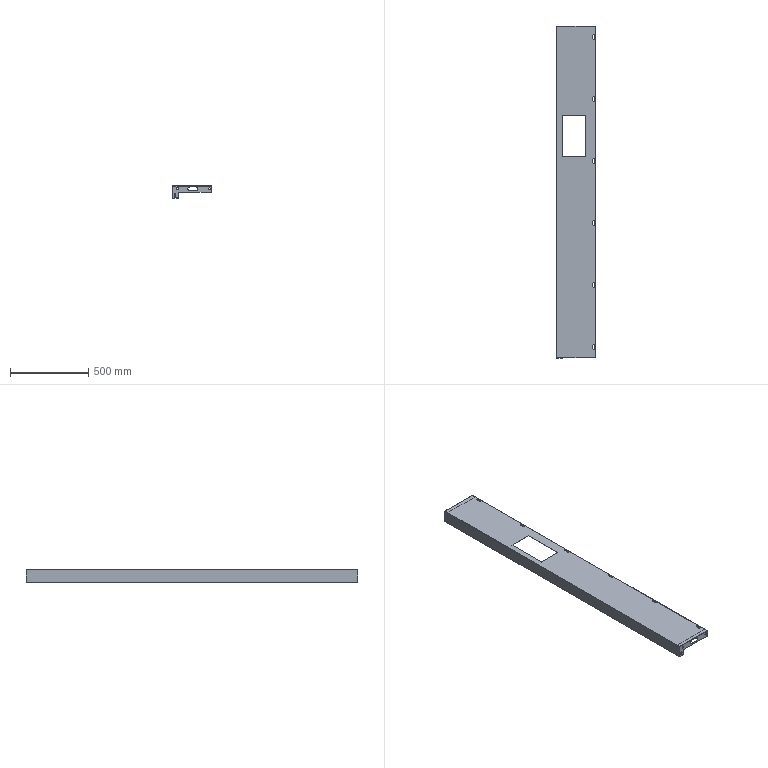Part | SolidWorks | features MirrorCompFeat 1, ReferencePattern 1 | 3 solids | 220 faces | box 250 x 2116 x 80 mm | volume 1096241 mm3 | plane 134 | cylinder 86 | commonest cylinder face diameters 6.2 x28 9 x18 11 x10 3.4 x9 10 x6 24 x6